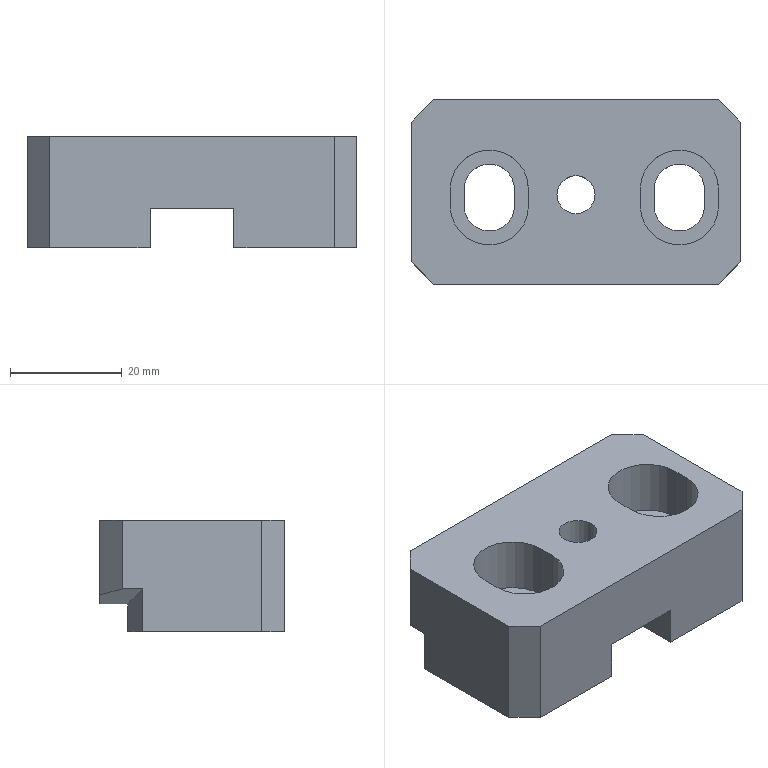Part | NX | features 20 2 | 1 solid | 41 faces | box 59 x 33 x 20 mm | volume 27333 mm3 | plane 32 | cylinder 9 | commonest cylinder face diameters 9 x4 14 x4 6.8 x1
STEP:
#1=CARTESIAN_POINT('',(2805.502,-433.5,16.5));
#2=VERTEX_POINT('',#1);
#3=CARTESIAN_POINT('',(2791.502,-433.5,16.5));
#4=VERTEX_POINT('',#3);
#5=CARTESIAN_POINT('',(2798.502,-433.5,16.5));
#6=DIRECTION('',(0.,0.,1.));
#7=DIRECTION('',(1.,0.,0.));
#8=AXIS2_PLACEMENT_3D('',#5,#6,#7);
#9=CIRCLE('',#8,7.);
#10=EDGE_CURVE('',#2,#4,#9,.T.);
#11=ORIENTED_EDGE('',*,*,#10,.F.);
#12=CARTESIAN_POINT('',(2805.502,-436.5,16.5));
#13=VERTEX_POINT('',#12);
#14=CARTESIAN_POINT('',(2805.502,-450.5,16.5));
#15=DIRECTION('',(0.,1.,0.));
#16=VECTOR('',#15,1000.);
#17=LINE('',#14,#16);
#18=EDGE_CURVE('',#13,#2,#17,.T.);
#19=ORIENTED_EDGE('',*,*,#18,.F.);
#20=CARTESIAN_POINT('',(2791.502,-436.5,16.5));
#21=VERTEX_POINT('',#20);
#22=CARTESIAN_POINT('',(2798.502,-436.5,16.5));
#23=DIRECTION('',(0.,0.,1.));
#24=DIRECTION('',(1.,0.,0.));
#25=AXIS2_PLACEMENT_3D('',#22,#23,#24);
#26=CIRCLE('',#25,7.);
#27=EDGE_CURVE('',#21,#13,#26,.T.);
#28=ORIENTED_EDGE('',*,*,#27,.F.);
#29=CARTESIAN_POINT('',(2791.502,-450.5,16.5));
#30=DIRECTION('',(0.,-1.,0.));
#31=VECTOR('',#30,1000.);
#32=LINE('',#29,#31);
#33=EDGE_CURVE('',#4,#21,#32,.T.);
#34=ORIENTED_EDGE('',*,*,#33,.F.);
#35=EDGE_LOOP('',(#11,#19,#28,#34));
#36=FACE_BOUND('',#35,.T.);
#37=CARTESIAN_POINT('',(2771.502,-436.5,16.5));
#38=VERTEX_POINT('',#37);
#39=CARTESIAN_POINT('',(2771.502,-433.5,16.5));
#40=VERTEX_POINT('',#39);
#41=CARTESIAN_POINT('',(2771.502,-450.5,16.5));
#42=DIRECTION('',(0.,1.,0.));
#43=VECTOR('',#42,1000.);
#44=LINE('',#41,#43);
#45=EDGE_CURVE('',#38,#40,#44,.T.);
#46=ORIENTED_EDGE('',*,*,#45,.F.);
#47=CARTESIAN_POINT('',(2757.502,-436.5,16.5));
#48=VERTEX_POINT('',#47);
#49=CARTESIAN_POINT('',(2764.502,-436.5,16.5));
#50=DIRECTION('',(0.,0.,1.));
#51=DIRECTION('',(1.,0.,0.));
#52=AXIS2_PLACEMENT_3D('',#49,#50,#51);
#53=CIRCLE('',#52,7.);
#54=EDGE_CURVE('',#48,#38,#53,.T.);
#55=ORIENTED_EDGE('',*,*,#54,.F.);
#56=CARTESIAN_POINT('',(2757.502,-433.5,16.5));
#57=VERTEX_POINT('',#56);
#58=CARTESIAN_POINT('',(2757.502,-450.5,16.5));
#59=DIRECTION('',(0.,-1.,0.));
#60=VECTOR('',#59,1000.);
#61=LINE('',#58,#60);
#62=EDGE_CURVE('',#57,#48,#61,.T.);
#63=ORIENTED_EDGE('',*,*,#62,.F.);
#64=CARTESIAN_POINT('',(2764.502,-433.5,16.5));
#65=DIRECTION('',(0.,0.,1.));
#66=DIRECTION('',(1.,0.,0.));
#67=AXIS2_PLACEMENT_3D('',#64,#65,#66);
#68=CIRCLE('',#67,7.);
#69=EDGE_CURVE('',#40,#57,#68,.T.);
#70=ORIENTED_EDGE('',*,*,#69,.F.);
#71=EDGE_LOOP('',(#46,#55,#63,#70));
#72=FACE_BOUND('',#71,.T.);
#73=CARTESIAN_POINT('',(2805.502,-417.5,16.5));
#74=VERTEX_POINT('',#73);
#75=CARTESIAN_POINT('',(2754.502,-417.5,16.5));
#76=VERTEX_POINT('',#75);
#77=CARTESIAN_POINT('',(2908.502,-417.5,16.5));
#78=DIRECTION('',(-1.,0.,0.));
#79=VECTOR('',#78,1000.);
#80=LINE('',#77,#79);
#81=EDGE_CURVE('',#74,#76,#80,.T.);
#82=ORIENTED_EDGE('',*,*,#81,.T.);
#83=CARTESIAN_POINT('',(2750.502,-421.5,16.5));
#84=VERTEX_POINT('',#83);
#85=CARTESIAN_POINT('',(2750.502,-421.5,16.5));
#86=DIRECTION('',(-0.7071,-0.7071,0.));
#87=VECTOR('',#86,1000.);
#88=LINE('',#85,#87);
#89=EDGE_CURVE('',#76,#84,#88,.T.);
#90=ORIENTED_EDGE('',*,*,#89,.T.);
#91=CARTESIAN_POINT('',(2750.502,-446.5,16.5));
#92=VERTEX_POINT('',#91);
#93=CARTESIAN_POINT('',(2750.502,-417.5,16.5));
#94=DIRECTION('',(0.,-1.,0.));
#95=VECTOR('',#94,1000.);
#96=LINE('',#93,#95);
#97=EDGE_CURVE('',#84,#92,#96,.T.);
#98=ORIENTED_EDGE('',*,*,#97,.T.);
#99=CARTESIAN_POINT('',(2754.502,-450.5,16.5));
#100=VERTEX_POINT('',#99);
#101=CARTESIAN_POINT('',(2754.502,-450.5,16.5));
#102=DIRECTION('',(0.7071,-0.7071,0.));
#103=VECTOR('',#102,1000.);
#104=LINE('',#101,#103);
#105=EDGE_CURVE('',#92,#100,#104,.T.);
#106=ORIENTED_EDGE('',*,*,#105,.T.);
#107=CARTESIAN_POINT('',(2805.502,-450.5,16.5));
#108=VERTEX_POINT('',#107);
#109=CARTESIAN_POINT('',(2828.502,-450.5,16.5));
#110=DIRECTION('',(1.,0.,0.));
#111=VECTOR('',#110,1000.);
#112=LINE('',#109,#111);
#113=EDGE_CURVE('',#100,#108,#112,.T.);
#114=ORIENTED_EDGE('',*,*,#113,.T.);
#115=CARTESIAN_POINT('',(2809.502,-446.5,16.5));
#116=VERTEX_POINT('',#115);
#117=CARTESIAN_POINT('',(2809.502,-446.5,16.5));
#118=DIRECTION('',(0.7071,0.7071,0.));
#119=VECTOR('',#118,1000.);
#120=LINE('',#117,#119);
#121=EDGE_CURVE('',#108,#116,#120,.T.);
#122=ORIENTED_EDGE('',*,*,#121,.T.);
#123=CARTESIAN_POINT('',(2809.502,-421.5,16.5));
#124=VERTEX_POINT('',#123);
#125=CARTESIAN_POINT('',(2809.502,-450.5,16.5));
#126=DIRECTION('',(0.,1.,0.));
#127=VECTOR('',#126,1000.);
#128=LINE('',#125,#127);
#129=EDGE_CURVE('',#116,#124,#128,.T.);
#130=ORIENTED_EDGE('',*,*,#129,.T.);
#131=CARTESIAN_POINT('',(2805.502,-417.5,16.5));
#132=DIRECTION('',(-0.7071,0.7071,0.));
#133=VECTOR('',#132,1000.);
#134=LINE('',#131,#133);
#135=EDGE_CURVE('',#124,#74,#134,.T.);
#136=ORIENTED_EDGE('',*,*,#135,.T.);
#137=EDGE_LOOP('',(#82,#90,#98,#106,#114,#122,#130,#136));
#138=FACE_BOUND('',#137,.T.);
#139=CARTESIAN_POINT('',(2783.402,-434.5,16.5));
#140=VERTEX_POINT('',#139);
#141=CARTESIAN_POINT('',(2780.002,-434.5,16.5));
#142=DIRECTION('',(0.,0.,-1.));
#143=DIRECTION('',(1.,0.,0.));
#144=AXIS2_PLACEMENT_3D('',#141,#142,#143);
#145=CIRCLE('',#144,3.4);
#146=EDGE_CURVE('',#140,#140,#145,.T.);
#147=ORIENTED_EDGE('',*,*,#146,.T.);
#148=EDGE_LOOP('',(#147));
#149=FACE_BOUND('',#148,.T.);
#150=CARTESIAN_POINT('',(2908.502,-450.5,16.5));
#151=DIRECTION('',(0.,0.,1.));
#152=DIRECTION('',(-1.,0.,0.));
#153=AXIS2_PLACEMENT_3D('',#150,#151,#152);
#154=PLANE('',#153);
#155=ADVANCED_FACE('',(#36,#72,#138,#149),#154,.T.);
#156=CARTESIAN_POINT('',(2787.502,-417.5,3.5));
#157=VERTEX_POINT('',#156);
#158=CARTESIAN_POINT('',(2787.502,-450.5,3.5));
#159=VERTEX_POINT('',#158);
#160=CARTESIAN_POINT('',(2787.502,-436.5,3.5));
#161=DIRECTION('',(0.,-1.,0.));
#162=VECTOR('',#161,1000.);
#163=LINE('',#160,#162);
#164=EDGE_CURVE('',#157,#159,#163,.T.);
#165=ORIENTED_EDGE('',*,*,#164,.F.);
#166=CARTESIAN_POINT('',(2787.502,-417.5,1.5));
#167=VERTEX_POINT('',#166);
#168=CARTESIAN_POINT('',(2787.502,-417.5,11.5));
#169=DIRECTION('',(0.,0.,-1.));
#170=VECTOR('',#169,1000.);
#171=LINE('',#168,#170);
#172=EDGE_CURVE('',#157,#167,#171,.T.);
#173=ORIENTED_EDGE('',*,*,#172,.T.);
#174=CARTESIAN_POINT('',(2787.502,-422.5,1.5));
#175=VERTEX_POINT('',#174);
#176=CARTESIAN_POINT('',(2787.502,-396.891,1.5));
#177=DIRECTION('',(0.,1.,0.));
#178=VECTOR('',#177,1000.);
#179=LINE('',#176,#178);
#180=EDGE_CURVE('',#175,#167,#179,.T.);
#181=ORIENTED_EDGE('',*,*,#180,.F.);
#182=CARTESIAN_POINT('',(2787.502,-422.5,-3.5));
#183=VERTEX_POINT('',#182);
#184=CARTESIAN_POINT('',(2787.502,-422.5,3.5));
#185=DIRECTION('',(0.,0.,-1.));
#186=VECTOR('',#185,1000.);
#187=LINE('',#184,#186);
#188=EDGE_CURVE('',#175,#183,#187,.T.);
#189=ORIENTED_EDGE('',*,*,#188,.T.);
#190=CARTESIAN_POINT('',(2787.502,-450.5,-3.5));
#191=VERTEX_POINT('',#190);
#192=CARTESIAN_POINT('',(2787.502,-450.5,-3.5));
#193=DIRECTION('',(0.,-1.,0.));
#194=VECTOR('',#193,1000.);
#195=LINE('',#192,#194);
#196=EDGE_CURVE('',#183,#191,#195,.T.);
#197=ORIENTED_EDGE('',*,*,#196,.T.);
#198=CARTESIAN_POINT('',(2787.502,-450.5,11.5));
#199=DIRECTION('',(0.,0.,1.));
#200=VECTOR('',#199,1000.);
#201=LINE('',#198,#200);
#202=EDGE_CURVE('',#191,#159,#201,.T.);
#203=ORIENTED_EDGE('',*,*,#202,.T.);
#204=EDGE_LOOP('',(#165,#173,#181,#189,#197,#203));
#205=FACE_BOUND('',#204,.T.);
#206=CARTESIAN_POINT('',(2787.502,-436.5,0.));
#207=DIRECTION('',(-1.,0.,0.));
#208=DIRECTION('',(0.,0.,1.));
#209=AXIS2_PLACEMENT_3D('',#206,#207,#208);
#210=PLANE('',#209);
#211=ADVANCED_FACE('',(#205),#210,.T.);
#212=CARTESIAN_POINT('',(2772.502,-422.5,-3.5));
#213=VERTEX_POINT('',#212);
#214=CARTESIAN_POINT('',(2772.502,-450.5,-3.5));
#215=VERTEX_POINT('',#214);
#216=CARTESIAN_POINT('',(2772.502,-450.5,-3.5));
#217=DIRECTION('',(0.,-1.,0.));
#218=VECTOR('',#217,1000.);
#219=LINE('',#216,#218);
#220=EDGE_CURVE('',#213,#215,#219,.T.);
#221=ORIENTED_EDGE('',*,*,#220,.F.);
#222=CARTESIAN_POINT('',(2772.502,-422.5,1.5));
#223=VERTEX_POINT('',#222);
#224=CARTESIAN_POINT('',(2772.502,-422.5,3.5));
#225=DIRECTION('',(0.,0.,-1.));
#226=VECTOR('',#225,1000.);
#227=LINE('',#224,#226);
#228=EDGE_CURVE('',#223,#213,#227,.T.);
#229=ORIENTED_EDGE('',*,*,#228,.F.);
#230=CARTESIAN_POINT('',(2772.502,-417.5,1.5));
#231=VERTEX_POINT('',#230);
#232=CARTESIAN_POINT('',(2772.502,-396.891,1.5));
#233=DIRECTION('',(0.,1.,0.));
#234=VECTOR('',#233,1000.);
#235=LINE('',#232,#234);
#236=EDGE_CURVE('',#223,#231,#235,.T.);
#237=ORIENTED_EDGE('',*,*,#236,.T.);
#238=CARTESIAN_POINT('',(2772.502,-417.5,3.5));
#239=VERTEX_POINT('',#238);
#240=CARTESIAN_POINT('',(2772.502,-417.5,11.5));
#241=DIRECTION('',(0.,0.,-1.));
#242=VECTOR('',#241,1000.);
#243=LINE('',#240,#242);
#244=EDGE_CURVE('',#239,#231,#243,.T.);
#245=ORIENTED_EDGE('',*,*,#244,.F.);
#246=CARTESIAN_POINT('',(2772.502,-450.5,3.5));
#247=VERTEX_POINT('',#246);
#248=CARTESIAN_POINT('',(2772.502,-436.5,3.5));
#249=DIRECTION('',(0.,1.,0.));
#250=VECTOR('',#249,1000.);
#251=LINE('',#248,#250);
#252=EDGE_CURVE('',#247,#239,#251,.T.);
#253=ORIENTED_EDGE('',*,*,#252,.F.);
#254=CARTESIAN_POINT('',(2772.502,-450.5,11.5));
#255=DIRECTION('',(0.,0.,1.));
#256=VECTOR('',#255,1000.);
#257=LINE('',#254,#256);
#258=EDGE_CURVE('',#215,#247,#257,.T.);
#259=ORIENTED_EDGE('',*,*,#258,.F.);
#260=EDGE_LOOP('',(#221,#229,#237,#245,#253,#259));
#261=FACE_BOUND('',#260,.T.);
#262=CARTESIAN_POINT('',(2772.502,-436.5,-9.5));
#263=DIRECTION('',(-1.,0.,0.));
#264=DIRECTION('',(0.,0.,-1.));
#265=AXIS2_PLACEMENT_3D('',#262,#263,#264);
#266=PLANE('',#265);
#267=ADVANCED_FACE('',(#261),#266,.F.);
#268=CARTESIAN_POINT('',(2783.402,-434.5,3.5));
#269=VERTEX_POINT('',#268);
#270=CARTESIAN_POINT('',(2780.002,-434.5,3.5));
#271=DIRECTION('',(0.,0.,1.));
#272=DIRECTION('',(1.,0.,0.));
#273=AXIS2_PLACEMENT_3D('',#270,#271,#272);
#274=CIRCLE('',#273,3.4);
#275=EDGE_CURVE('',#269,#269,#274,.T.);
#276=ORIENTED_EDGE('',*,*,#275,.T.);
#277=EDGE_LOOP('',(#276));
#278=FACE_BOUND('',#277,.T.);
#279=CARTESIAN_POINT('',(2850.502,-450.5,3.5));
#280=DIRECTION('',(1.,0.,0.));
#281=VECTOR('',#280,1000.);
#282=LINE('',#279,#281);
#283=EDGE_CURVE('',#247,#159,#282,.T.);
#284=ORIENTED_EDGE('',*,*,#283,.F.);
#285=ORIENTED_EDGE('',*,*,#252,.T.);
#286=CARTESIAN_POINT('',(2930.502,-417.5,3.5));
#287=DIRECTION('',(-1.,0.,0.));
#288=VECTOR('',#287,1000.);
#289=LINE('',#286,#288);
#290=EDGE_CURVE('',#157,#239,#289,.T.);
#291=ORIENTED_EDGE('',*,*,#290,.F.);
#292=ORIENTED_EDGE('',*,*,#164,.T.);
#293=EDGE_LOOP('',(#284,#285,#291,#292));
#294=FACE_BOUND('',#293,.T.);
#295=CARTESIAN_POINT('',(2780.002,-436.5,3.5));
#296=DIRECTION('',(0.,0.,1.));
#297=DIRECTION('',(0.,-1.,0.));
#298=AXIS2_PLACEMENT_3D('',#295,#296,#297);
#299=PLANE('',#298);
#300=ADVANCED_FACE('',(#278,#294),#299,.F.);
#301=CARTESIAN_POINT('',(2794.002,-436.5,6.5));
#302=VERTEX_POINT('',#301);
#303=CARTESIAN_POINT('',(2794.002,-433.5,6.5));
#304=VERTEX_POINT('',#303);
#305=CARTESIAN_POINT('',(2794.002,-432.5,6.5));
#306=DIRECTION('',(0.,1.,0.));
#307=VECTOR('',#306,1000.);
#308=LINE('',#305,#307);
#309=EDGE_CURVE('',#302,#304,#308,.T.);
#310=ORIENTED_EDGE('',*,*,#309,.T.);
#311=CARTESIAN_POINT('',(2803.002,-433.5,6.5));
#312=VERTEX_POINT('',#311);
#313=CARTESIAN_POINT('',(2798.502,-433.5,6.5));
#314=DIRECTION('',(0.,0.,-1.));
#315=DIRECTION('',(-1.,0.,0.));
#316=AXIS2_PLACEMENT_3D('',#313,#314,#315);
#317=CIRCLE('',#316,4.5);
#318=EDGE_CURVE('',#304,#312,#317,.T.);
#319=ORIENTED_EDGE('',*,*,#318,.T.);
#320=CARTESIAN_POINT('',(2803.002,-436.5,6.5));
#321=VERTEX_POINT('',#320);
#322=CARTESIAN_POINT('',(2803.002,-439.5,6.5));
#323=DIRECTION('',(0.,-1.,0.));
#324=VECTOR('',#323,1000.);
#325=LINE('',#322,#324);
#326=EDGE_CURVE('',#312,#321,#325,.T.);
#327=ORIENTED_EDGE('',*,*,#326,.T.);
#328=CARTESIAN_POINT('',(2798.502,-436.5,6.5));
#329=DIRECTION('',(0.,0.,-1.));
#330=DIRECTION('',(-1.,0.,0.));
#331=AXIS2_PLACEMENT_3D('',#328,#329,#330);
#332=CIRCLE('',#331,4.5);
#333=EDGE_CURVE('',#321,#302,#332,.T.);
#334=ORIENTED_EDGE('',*,*,#333,.T.);
#335=EDGE_LOOP('',(#310,#319,#327,#334));
#336=FACE_BOUND('',#335,.T.);
#337=CARTESIAN_POINT('',(2805.502,-433.5,6.5));
#338=VERTEX_POINT('',#337);
#339=CARTESIAN_POINT('',(2791.502,-433.5,6.5));
#340=VERTEX_POINT('',#339);
#341=CARTESIAN_POINT('',(2798.502,-433.5,6.5));
#342=DIRECTION('',(0.,0.,1.));
#343=DIRECTION('',(-1.,0.,0.));
#344=AXIS2_PLACEMENT_3D('',#341,#342,#343);
#345=CIRCLE('',#344,7.);
#346=EDGE_CURVE('',#338,#340,#345,.T.);
#347=ORIENTED_EDGE('',*,*,#346,.T.);
#348=CARTESIAN_POINT('',(2791.502,-436.5,6.5));
#349=VERTEX_POINT('',#348);
#350=CARTESIAN_POINT('',(2791.502,-439.5,6.5));
#351=DIRECTION('',(0.,-1.,0.));
#352=VECTOR('',#351,1000.);
#353=LINE('',#350,#352);
#354=EDGE_CURVE('',#340,#349,#353,.T.);
#355=ORIENTED_EDGE('',*,*,#354,.T.);
#356=CARTESIAN_POINT('',(2805.502,-436.5,6.5));
#357=VERTEX_POINT('',#356);
#358=CARTESIAN_POINT('',(2798.502,-436.5,6.5));
#359=DIRECTION('',(0.,0.,1.));
#360=DIRECTION('',(-1.,0.,0.));
#361=AXIS2_PLACEMENT_3D('',#358,#359,#360);
#362=CIRCLE('',#361,7.);
#363=EDGE_CURVE('',#349,#357,#362,.T.);
#364=ORIENTED_EDGE('',*,*,#363,.T.);
#365=CARTESIAN_POINT('',(2805.502,-432.5,6.5));
#366=DIRECTION('',(0.,1.,0.));
#367=VECTOR('',#366,1000.);
#368=LINE('',#365,#367);
#369=EDGE_CURVE('',#357,#338,#368,.T.);
#370=ORIENTED_EDGE('',*,*,#369,.T.);
#371=EDGE_LOOP('',(#347,#355,#364,#370));
#372=FACE_BOUND('',#371,.T.);
#373=CARTESIAN_POINT('',(2798.502,-432.5,6.5));
#374=DIRECTION('',(0.,0.,-1.));
#375=DIRECTION('',(1.,0.,0.));
#376=AXIS2_PLACEMENT_3D('',#373,#374,#375);
#377=PLANE('',#376);
#378=ADVANCED_FACE('',(#336,#372),#377,.F.);
#379=CARTESIAN_POINT('',(2799.502,-417.5,1.5));
#380=VERTEX_POINT('',#379);
#381=CARTESIAN_POINT('',(2799.502,-422.5,1.5));
#382=VERTEX_POINT('',#381);
#383=CARTESIAN_POINT('',(2799.502,-425.18,1.5));
#384=DIRECTION('',(0.,-1.,0.));
#385=VECTOR('',#384,1000.);
#386=LINE('',#383,#385);
#387=EDGE_CURVE('',#380,#382,#386,.T.);
#388=ORIENTED_EDGE('',*,*,#387,.F.);
#389=CARTESIAN_POINT('',(2805.502,-417.5,3.108));
#390=VERTEX_POINT('',#389);
#391=CARTESIAN_POINT('',(2799.502,-417.5,1.5));
#392=DIRECTION('',(-0.9659,0.,-0.2588));
#393=VECTOR('',#392,1000.);
#394=LINE('',#391,#393);
#395=EDGE_CURVE('',#390,#380,#394,.T.);
#396=ORIENTED_EDGE('',*,*,#395,.F.);
#397=CARTESIAN_POINT('',(2809.502,-421.5,4.179));
#398=VERTEX_POINT('',#397);
#399=CARTESIAN_POINT('',(2792.451,-404.449,-0.3894));
#400=DIRECTION('',(0.6947,-0.6947,0.1862));
#401=VECTOR('',#400,1000.);
#402=LINE('',#399,#401);
#403=EDGE_CURVE('',#390,#398,#402,.T.);
#404=ORIENTED_EDGE('',*,*,#403,.T.);
#405=CARTESIAN_POINT('',(2809.502,-425.18,4.179));
#406=VERTEX_POINT('',#405);
#407=CARTESIAN_POINT('',(2809.502,-417.5,4.179));
#408=DIRECTION('',(0.,1.,0.));
#409=VECTOR('',#408,1000.);
#410=LINE('',#407,#409);
#411=EDGE_CURVE('',#406,#398,#410,.T.);
#412=ORIENTED_EDGE('',*,*,#411,.F.);
#413=CARTESIAN_POINT('',(2808.875,-425.012,4.011));
#414=DIRECTION('',(0.9351,-0.2506,0.2506));
#415=VECTOR('',#414,1000.);
#416=LINE('',#413,#415);
#417=EDGE_CURVE('',#382,#406,#416,.T.);
#418=ORIENTED_EDGE('',*,*,#417,.F.);
#419=EDGE_LOOP('',(#388,#396,#404,#412,#418));
#420=FACE_BOUND('',#419,.T.);
#421=CARTESIAN_POINT('',(2799.502,-396.891,1.5));
#422=DIRECTION('',(0.2588,0.,-0.9659));
#423=DIRECTION('',(0.9659,0.,0.2588));
#424=AXIS2_PLACEMENT_3D('',#421,#422,#423);
#425=PLANE('',#424);
#426=ADVANCED_FACE('',(#420),#425,.T.);
#427=CARTESIAN_POINT('',(2769.002,-433.5,6.5));
#428=VERTEX_POINT('',#427);
#429=CARTESIAN_POINT('',(2769.002,-436.5,6.5));
#430=VERTEX_POINT('',#429);
#431=CARTESIAN_POINT('',(2769.002,-432.5,6.5));
#432=DIRECTION('',(0.,-1.,0.));
#433=VECTOR('',#432,1000.);
#434=LINE('',#431,#433);
#435=EDGE_CURVE('',#428,#430,#434,.T.);
#436=ORIENTED_EDGE('',*,*,#435,.T.);
#437=CARTESIAN_POINT('',(2760.002,-436.5,6.5));
#438=VERTEX_POINT('',#437);
#439=CARTESIAN_POINT('',(2764.502,-436.5,6.5));
#440=DIRECTION('',(0.,0.,-1.));
#441=DIRECTION('',(-1.,0.,0.));
#442=AXIS2_PLACEMENT_3D('',#439,#440,#441);
#443=CIRCLE('',#442,4.5);
#444=EDGE_CURVE('',#430,#438,#443,.T.);
#445=ORIENTED_EDGE('',*,*,#444,.T.);
#446=CARTESIAN_POINT('',(2760.002,-433.5,6.5));
#447=VERTEX_POINT('',#446);
#448=CARTESIAN_POINT('',(2760.002,-439.5,6.5));
#449=DIRECTION('',(0.,1.,0.));
#450=VECTOR('',#449,1000.);
#451=LINE('',#448,#450);
#452=EDGE_CURVE('',#438,#447,#451,.T.);
#453=ORIENTED_EDGE('',*,*,#452,.T.);
#454=CARTESIAN_POINT('',(2764.502,-433.5,6.5));
#455=DIRECTION('',(0.,0.,-1.));
#456=DIRECTION('',(-1.,0.,0.));
#457=AXIS2_PLACEMENT_3D('',#454,#455,#456);
#458=CIRCLE('',#457,4.5);
#459=EDGE_CURVE('',#447,#428,#458,.T.);
#460=ORIENTED_EDGE('',*,*,#459,.T.);
#461=EDGE_LOOP('',(#436,#445,#453,#460));
#462=FACE_BOUND('',#461,.T.);
#463=CARTESIAN_POINT('',(2771.502,-433.5,6.5));
#464=VERTEX_POINT('',#463);
#465=CARTESIAN_POINT('',(2757.502,-433.5,6.5));
#466=VERTEX_POINT('',#465);
#467=CARTESIAN_POINT('',(2764.502,-433.5,6.5));
#468=DIRECTION('',(0.,0.,1.));
#469=DIRECTION('',(-1.,0.,0.));
#470=AXIS2_PLACEMENT_3D('',#467,#468,#469);
#471=CIRCLE('',#470,7.);
#472=EDGE_CURVE('',#464,#466,#471,.T.);
#473=ORIENTED_EDGE('',*,*,#472,.T.);
#474=CARTESIAN_POINT('',(2757.502,-436.5,6.5));
#475=VERTEX_POINT('',#474);
#476=CARTESIAN_POINT('',(2757.502,-432.5,6.5));
#477=DIRECTION('',(0.,-1.,0.));
#478=VECTOR('',#477,1000.);
#479=LINE('',#476,#478);
#480=EDGE_CURVE('',#466,#475,#479,.T.);
#481=ORIENTED_EDGE('',*,*,#480,.T.);
#482=CARTESIAN_POINT('',(2771.502,-436.5,6.5));
#483=VERTEX_POINT('',#482);
#484=CARTESIAN_POINT('',(2764.502,-436.5,6.5));
#485=DIRECTION('',(0.,0.,1.));
#486=DIRECTION('',(-1.,0.,0.));
#487=AXIS2_PLACEMENT_3D('',#484,#485,#486);
#488=CIRCLE('',#487,7.);
#489=EDGE_CURVE('',#475,#483,#488,.T.);
#490=ORIENTED_EDGE('',*,*,#489,.T.);
#491=CARTESIAN_POINT('',(2771.502,-439.5,6.5));
#492=DIRECTION('',(0.,1.,0.));
#493=VECTOR('',#492,1000.);
#494=LINE('',#491,#493);
#495=EDGE_CURVE('',#483,#464,#494,.T.);
#496=ORIENTED_EDGE('',*,*,#495,.T.);
#497=EDGE_LOOP('',(#473,#481,#490,#496));
#498=FACE_BOUND('',#497,.T.);
#499=CARTESIAN_POINT('',(2764.502,-432.5,6.5));
#500=DIRECTION('',(0.,0.,-1.));
#501=DIRECTION('',(-1.,0.,0.));
#502=AXIS2_PLACEMENT_3D('',#499,#500,#501);
#503=PLANE('',#502);
#504=ADVANCED_FACE('',(#462,#498),#503,.F.);
#505=ORIENTED_EDGE('',*,*,#33,.T.);
#506=CARTESIAN_POINT('',(2791.502,-436.5,42.5));
#507=DIRECTION('',(0.,0.,1.));
#508=VECTOR('',#507,1000.);
#509=LINE('',#506,#508);
#510=EDGE_CURVE('',#349,#21,#509,.T.);
#511=ORIENTED_EDGE('',*,*,#510,.F.);
#512=ORIENTED_EDGE('',*,*,#354,.F.);
#513=CARTESIAN_POINT('',(2791.502,-433.5,42.5));
#514=DIRECTION('',(0.,0.,1.));
#515=VECTOR('',#514,1000.);
#516=LINE('',#513,#515);
#517=EDGE_CURVE('',#340,#4,#516,.T.);
#518=ORIENTED_EDGE('',*,*,#517,.T.);
#519=EDGE_LOOP('',(#505,#511,#512,#518));
#520=FACE_BOUND('',#519,.T.);
#521=CARTESIAN_POINT('',(2791.502,-439.5,42.5));
#522=DIRECTION('',(-1.,0.,0.));
#523=DIRECTION('',(0.,0.,-1.));
#524=AXIS2_PLACEMENT_3D('',#521,#522,#523);
#525=PLANE('',#524);
#526=ADVANCED_FACE('',(#520),#525,.F.);
#527=ORIENTED_EDGE('',*,*,#27,.T.);
#528=CARTESIAN_POINT('',(2805.502,-436.5,42.5));
#529=DIRECTION('',(0.,0.,1.));
#530=VECTOR('',#529,1000.);
#531=LINE('',#528,#530);
#532=EDGE_CURVE('',#357,#13,#531,.T.);
#533=ORIENTED_EDGE('',*,*,#532,.F.);
#534=ORIENTED_EDGE('',*,*,#363,.F.);
#535=ORIENTED_EDGE('',*,*,#510,.T.);
#536=EDGE_LOOP('',(#527,#533,#534,#535));
#537=FACE_BOUND('',#536,.T.);
#538=CARTESIAN_POINT('',(2798.502,-436.5,42.5));
#539=DIRECTION('',(0.,0.,-1.));
#540=DIRECTION('',(1.,0.,0.));
#541=AXIS2_PLACEMENT_3D('',#538,#539,#540);
#542=CYLINDRICAL_SURFACE('',#541,7.);
#543=ADVANCED_FACE('',(#537),#542,.F.);
#544=ORIENTED_EDGE('',*,*,#18,.T.);
#545=CARTESIAN_POINT('',(2805.502,-433.5,42.5));
#546=DIRECTION('',(0.,0.,1.));
#547=VECTOR('',#546,1000.);
#548=LINE('',#545,#547);
#549=EDGE_CURVE('',#338,#2,#548,.T.);
#550=ORIENTED_EDGE('',*,*,#549,.F.);
#551=ORIENTED_EDGE('',*,*,#369,.F.);
#552=ORIENTED_EDGE('',*,*,#532,.T.);
#553=EDGE_LOOP('',(#544,#550,#551,#552));
#554=FACE_BOUND('',#553,.T.);
#555=CARTESIAN_POINT('',(2805.502,-432.5,42.5));
#556=DIRECTION('',(1.,0.,0.));
#557=DIRECTION('',(0.,0.,1.));
#558=AXIS2_PLACEMENT_3D('',#555,#556,#557);
#559=PLANE('',#558);
#560=ADVANCED_FACE('',(#554),#559,.F.);
#561=ORIENTED_EDGE('',*,*,#10,.T.);
#562=ORIENTED_EDGE('',*,*,#517,.F.);
#563=ORIENTED_EDGE('',*,*,#346,.F.);
#564=ORIENTED_EDGE('',*,*,#549,.T.);
#565=EDGE_LOOP('',(#561,#562,#563,#564));
#566=FACE_BOUND('',#565,.T.);
#567=CARTESIAN_POINT('',(2798.502,-433.5,42.5));
#568=DIRECTION('',(0.,0.,-1.));
#569=DIRECTION('',(1.,0.,0.));
#570=AXIS2_PLACEMENT_3D('',#567,#568,#569);
#571=CYLINDRICAL_SURFACE('',#570,7.);
#572=ADVANCED_FACE('',(#566),#571,.F.);
#573=ORIENTED_EDGE('',*,*,#135,.F.);
#574=CARTESIAN_POINT('',(2809.502,-421.5,11.5));
#575=DIRECTION('',(0.,0.,1.));
#576=VECTOR('',#575,1000.);
#577=LINE('',#574,#576);
#578=EDGE_CURVE('',#398,#124,#577,.T.);
#579=ORIENTED_EDGE('',*,*,#578,.F.);
#580=ORIENTED_EDGE('',*,*,#403,.F.);
#581=CARTESIAN_POINT('',(2805.502,-417.5,11.5));
#582=DIRECTION('',(0.,0.,-1.));
#583=VECTOR('',#582,1000.);
#584=LINE('',#581,#583);
#585=EDGE_CURVE('',#74,#390,#584,.T.);
#586=ORIENTED_EDGE('',*,*,#585,.F.);
#587=EDGE_LOOP('',(#573,#579,#580,#586));
#588=FACE_BOUND('',#587,.T.);
#589=CARTESIAN_POINT('',(2805.502,-417.5,11.5));
#590=DIRECTION('',(-0.7071,-0.7071,0.));
#591=DIRECTION('',(0.,0.,-1.));
#592=AXIS2_PLACEMENT_3D('',#589,#590,#591);
#593=PLANE('',#592);
#594=ADVANCED_FACE('',(#588),#593,.F.);
#595=ORIENTED_EDGE('',*,*,#69,.T.);
#596=CARTESIAN_POINT('',(2757.502,-433.5,42.5));
#597=DIRECTION('',(0.,0.,-1.));
#598=VECTOR('',#597,1000.);
#599=LINE('',#596,#598);
#600=EDGE_CURVE('',#57,#466,#599,.T.);
#601=ORIENTED_EDGE('',*,*,#600,.T.);
#602=ORIENTED_EDGE('',*,*,#472,.F.);
#603=CARTESIAN_POINT('',(2771.502,-433.5,42.5));
#604=DIRECTION('',(0.,0.,-1.));
#605=VECTOR('',#604,1000.);
#606=LINE('',#603,#605);
#607=EDGE_CURVE('',#40,#464,#606,.T.);
#608=ORIENTED_EDGE('',*,*,#607,.F.);
#609=EDGE_LOOP('',(#595,#601,#602,#608));
#610=FACE_BOUND('',#609,.T.);
#611=CARTESIAN_POINT('',(2764.502,-433.5,42.5));
#612=DIRECTION('',(0.,0.,-1.));
#613=DIRECTION('',(-1.,0.,0.));
#614=AXIS2_PLACEMENT_3D('',#611,#612,#613);
#615=CYLINDRICAL_SURFACE('',#614,7.);
#616=ADVANCED_FACE('',(#610),#615,.F.);
#617=ORIENTED_EDGE('',*,*,#62,.T.);
#618=CARTESIAN_POINT('',(2757.502,-436.5,42.5));
#619=DIRECTION('',(0.,0.,-1.));
#620=VECTOR('',#619,1000.);
#621=LINE('',#618,#620);
#622=EDGE_CURVE('',#48,#475,#621,.T.);
#623=ORIENTED_EDGE('',*,*,#622,.T.);
#624=ORIENTED_EDGE('',*,*,#480,.F.);
#625=ORIENTED_EDGE('',*,*,#600,.F.);
#626=EDGE_LOOP('',(#617,#623,#624,#625));
#627=FACE_BOUND('',#626,.T.);
#628=CARTESIAN_POINT('',(2757.502,-432.5,42.5));
#629=DIRECTION('',(-1.,0.,0.));
#630=DIRECTION('',(0.,0.,1.));
#631=AXIS2_PLACEMENT_3D('',#628,#629,#630);
#632=PLANE('',#631);
#633=ADVANCED_FACE('',(#627),#632,.F.);
#634=ORIENTED_EDGE('',*,*,#54,.T.);
#635=CARTESIAN_POINT('',(2771.502,-436.5,42.5));
#636=DIRECTION('',(0.,0.,-1.));
#637=VECTOR('',#636,1000.);
#638=LINE('',#635,#637);
#639=EDGE_CURVE('',#38,#483,#638,.T.);
#640=ORIENTED_EDGE('',*,*,#639,.T.);
#641=ORIENTED_EDGE('',*,*,#489,.F.);
#642=ORIENTED_EDGE('',*,*,#622,.F.);
#643=EDGE_LOOP('',(#634,#640,#641,#642));
#644=FACE_BOUND('',#643,.T.);
#645=CARTESIAN_POINT('',(2764.502,-436.5,42.5));
#646=DIRECTION('',(0.,0.,-1.));
#647=DIRECTION('',(-1.,0.,0.));
#648=AXIS2_PLACEMENT_3D('',#645,#646,#647);
#649=CYLINDRICAL_SURFACE('',#648,7.);
#650=ADVANCED_FACE('',(#644),#649,.F.);
#651=ORIENTED_EDGE('',*,*,#45,.T.);
#652=ORIENTED_EDGE('',*,*,#607,.T.);
#653=ORIENTED_EDGE('',*,*,#495,.F.);
#654=ORIENTED_EDGE('',*,*,#639,.F.);
#655=EDGE_LOOP('',(#651,#652,#653,#654));
#656=FACE_BOUND('',#655,.T.);
#657=CARTESIAN_POINT('',(2771.502,-439.5,42.5));
#658=DIRECTION('',(1.,0.,0.));
#659=DIRECTION('',(0.,0.,-1.));
#660=AXIS2_PLACEMENT_3D('',#657,#658,#659);
#661=PLANE('',#660);
#662=ADVANCED_FACE('',(#656),#661,.F.);
#663=ORIENTED_EDGE('',*,*,#411,.T.);
#664=ORIENTED_EDGE('',*,*,#578,.T.);
#665=ORIENTED_EDGE('',*,*,#129,.F.);
#666=CARTESIAN_POINT('',(2809.502,-446.5,-3.5));
#667=VERTEX_POINT('',#666);
#668=CARTESIAN_POINT('',(2809.502,-446.5,11.5));
#669=DIRECTION('',(0.,0.,-1.));
#670=VECTOR('',#669,1000.);
#671=LINE('',#668,#670);
#672=EDGE_CURVE('',#116,#667,#671,.T.);
#673=ORIENTED_EDGE('',*,*,#672,.T.);
#674=CARTESIAN_POINT('',(2809.502,-425.18,-3.5));
#675=VERTEX_POINT('',#674);
#676=CARTESIAN_POINT('',(2809.502,-450.5,-3.5));
#677=DIRECTION('',(0.,1.,0.));
#678=VECTOR('',#677,1000.);
#679=LINE('',#676,#678);
#680=EDGE_CURVE('',#667,#675,#679,.T.);
#681=ORIENTED_EDGE('',*,*,#680,.T.);
#682=CARTESIAN_POINT('',(2809.502,-425.18,3.5));
#683=DIRECTION('',(0.,0.,-1.));
#684=VECTOR('',#683,1000.);
#685=LINE('',#682,#684);
#686=EDGE_CURVE('',#406,#675,#685,.T.);
#687=ORIENTED_EDGE('',*,*,#686,.F.);
#688=EDGE_LOOP('',(#663,#664,#665,#673,#681,#687));
#689=FACE_BOUND('',#688,.T.);
#690=CARTESIAN_POINT('',(2809.502,-450.5,11.5));
#691=DIRECTION('',(-1.,0.,0.));
#692=DIRECTION('',(0.,0.,-1.));
#693=AXIS2_PLACEMENT_3D('',#690,#691,#692);
#694=PLANE('',#693);
#695=ADVANCED_FACE('',(#689),#694,.F.);
#696=CARTESIAN_POINT('',(2799.501,-422.5,1.5));
#697=VERTEX_POINT('',#696);
#698=CARTESIAN_POINT('',(2809.502,-425.18,1.5));
#699=DIRECTION('',(0.9659,-0.2588,0.));
#700=VECTOR('',#699,1000.);
#701=LINE('',#698,#700);
#702=EDGE_CURVE('',#697,#382,#701,.T.);
#703=ORIENTED_EDGE('',*,*,#702,.T.);
#704=ORIENTED_EDGE('',*,*,#417,.T.);
#705=ORIENTED_EDGE('',*,*,#686,.T.);
#706=CARTESIAN_POINT('',(2799.501,-422.5,-3.5));
#707=VERTEX_POINT('',#706);
#708=CARTESIAN_POINT('',(2809.502,-425.18,-3.5));
#709=DIRECTION('',(-0.9659,0.2588,0.));
#710=VECTOR('',#709,1000.);
#711=LINE('',#708,#710);
#712=EDGE_CURVE('',#675,#707,#711,.T.);
#713=ORIENTED_EDGE('',*,*,#712,.T.);
#714=CARTESIAN_POINT('',(2799.501,-422.5,3.5));
#715=DIRECTION('',(0.,0.,1.));
#716=VECTOR('',#715,1000.);
#717=LINE('',#714,#716);
#718=EDGE_CURVE('',#707,#697,#717,.T.);
#719=ORIENTED_EDGE('',*,*,#718,.T.);
#720=EDGE_LOOP('',(#703,#704,#705,#713,#719));
#721=FACE_BOUND('',#720,.T.);
#722=CARTESIAN_POINT('',(2809.502,-425.18,3.5));
#723=DIRECTION('',(-0.2588,-0.9659,0.));
#724=DIRECTION('',(0.9659,-0.2588,0.));
#725=AXIS2_PLACEMENT_3D('',#722,#723,#724);
#726=PLANE('',#725);
#727=ADVANCED_FACE('',(#721),#726,.F.);
#728=ORIENTED_EDGE('',*,*,#318,.F.);
#729=CARTESIAN_POINT('',(2794.002,-433.5,-3.5));
#730=VERTEX_POINT('',#729);
#731=CARTESIAN_POINT('',(2794.002,-433.5,42.5));
#732=DIRECTION('',(0.,0.,1.));
#733=VECTOR('',#732,1000.);
#734=LINE('',#731,#733);
#735=EDGE_CURVE('',#730,#304,#734,.T.);
#736=ORIENTED_EDGE('',*,*,#735,.F.);
#737=CARTESIAN_POINT('',(2803.002,-433.5,-3.5));
#738=VERTEX_POINT('',#737);
#739=CARTESIAN_POINT('',(2798.502,-433.5,-3.5));
#740=DIRECTION('',(0.,0.,1.));
#741=DIRECTION('',(1.,0.,0.));
#742=AXIS2_PLACEMENT_3D('',#739,#740,#741);
#743=CIRCLE('',#742,4.5);
#744=EDGE_CURVE('',#738,#730,#743,.T.);
#745=ORIENTED_EDGE('',*,*,#744,.F.);
#746=CARTESIAN_POINT('',(2803.002,-433.5,42.5));
#747=DIRECTION('',(0.,0.,1.));
#748=VECTOR('',#747,1000.);
#749=LINE('',#746,#748);
#750=EDGE_CURVE('',#738,#312,#749,.T.);
#751=ORIENTED_EDGE('',*,*,#750,.T.);
#752=EDGE_LOOP('',(#728,#736,#745,#751));
#753=FACE_BOUND('',#752,.T.);
#754=CARTESIAN_POINT('',(2798.502,-433.5,42.5));
#755=DIRECTION('',(0.,0.,-1.));
#756=DIRECTION('',(1.,0.,0.));
#757=AXIS2_PLACEMENT_3D('',#754,#755,#756);
#758=CYLINDRICAL_SURFACE('',#757,4.5);
#759=ADVANCED_FACE('',(#753),#758,.F.);
#760=ORIENTED_EDGE('',*,*,#326,.F.);
#761=ORIENTED_EDGE('',*,*,#750,.F.);
#762=CARTESIAN_POINT('',(2803.002,-436.5,-3.5));
#763=VERTEX_POINT('',#762);
#764=CARTESIAN_POINT('',(2803.002,-439.5,-3.5));
#765=DIRECTION('',(0.,1.,0.));
#766=VECTOR('',#765,1000.);
#767=LINE('',#764,#766);
#768=EDGE_CURVE('',#763,#738,#767,.T.);
#769=ORIENTED_EDGE('',*,*,#768,.F.);
#770=CARTESIAN_POINT('',(2803.002,-436.5,42.5));
#771=DIRECTION('',(0.,0.,1.));
#772=VECTOR('',#771,1000.);
#773=LINE('',#770,#772);
#774=EDGE_CURVE('',#763,#321,#773,.T.);
#775=ORIENTED_EDGE('',*,*,#774,.T.);
#776=EDGE_LOOP('',(#760,#761,#769,#775));
#777=FACE_BOUND('',#776,.T.);
#778=CARTESIAN_POINT('',(2803.002,-439.5,42.5));
#779=DIRECTION('',(-1.,0.,0.));
#780=DIRECTION('',(0.,0.,-1.));
#781=AXIS2_PLACEMENT_3D('',#778,#779,#780);
#782=PLANE('',#781);
#783=ADVANCED_FACE('',(#777),#782,.T.);
#784=ORIENTED_EDGE('',*,*,#333,.F.);
#785=ORIENTED_EDGE('',*,*,#774,.F.);
#786=CARTESIAN_POINT('',(2794.002,-436.5,-3.5));
#787=VERTEX_POINT('',#786);
#788=CARTESIAN_POINT('',(2798.502,-436.5,-3.5));
#789=DIRECTION('',(0.,0.,1.));
#790=DIRECTION('',(1.,0.,0.));
#791=AXIS2_PLACEMENT_3D('',#788,#789,#790);
#792=CIRCLE('',#791,4.5);
#793=EDGE_CURVE('',#787,#763,#792,.T.);
#794=ORIENTED_EDGE('',*,*,#793,.F.);
#795=CARTESIAN_POINT('',(2794.002,-436.5,42.5));
#796=DIRECTION('',(0.,0.,1.));
#797=VECTOR('',#796,1000.);
#798=LINE('',#795,#797);
#799=EDGE_CURVE('',#787,#302,#798,.T.);
#800=ORIENTED_EDGE('',*,*,#799,.T.);
#801=EDGE_LOOP('',(#784,#785,#794,#800));
#802=FACE_BOUND('',#801,.T.);
#803=CARTESIAN_POINT('',(2798.502,-436.5,42.5));
#804=DIRECTION('',(0.,0.,-1.));
#805=DIRECTION('',(1.,0.,0.));
#806=AXIS2_PLACEMENT_3D('',#803,#804,#805);
#807=CYLINDRICAL_SURFACE('',#806,4.5);
#808=ADVANCED_FACE('',(#802),#807,.F.);
#809=ORIENTED_EDGE('',*,*,#309,.F.);
#810=ORIENTED_EDGE('',*,*,#799,.F.);
#811=CARTESIAN_POINT('',(2794.002,-432.5,-3.5));
#812=DIRECTION('',(0.,-1.,0.));
#813=VECTOR('',#812,1000.);
#814=LINE('',#811,#813);
#815=EDGE_CURVE('',#730,#787,#814,.T.);
#816=ORIENTED_EDGE('',*,*,#815,.F.);
#817=ORIENTED_EDGE('',*,*,#735,.T.);
#818=EDGE_LOOP('',(#809,#810,#816,#817));
#819=FACE_BOUND('',#818,.T.);
#820=CARTESIAN_POINT('',(2794.002,-432.5,42.5));
#821=DIRECTION('',(1.,0.,0.));
#822=DIRECTION('',(0.,0.,1.));
#823=AXIS2_PLACEMENT_3D('',#820,#821,#822);
#824=PLANE('',#823);
#825=ADVANCED_FACE('',(#819),#824,.T.);
#826=ORIENTED_EDGE('',*,*,#395,.T.);
#827=CARTESIAN_POINT('',(2870.773,-417.5,1.5));
#828=DIRECTION('',(1.,0.,0.));
#829=VECTOR('',#828,1000.);
#830=LINE('',#827,#829);
#831=EDGE_CURVE('',#167,#380,#830,.T.);
#832=ORIENTED_EDGE('',*,*,#831,.F.);
#833=ORIENTED_EDGE('',*,*,#172,.F.);
#834=ORIENTED_EDGE('',*,*,#290,.T.);
#835=ORIENTED_EDGE('',*,*,#244,.T.);
#836=CARTESIAN_POINT('',(2760.502,-417.5,1.5));
#837=VERTEX_POINT('',#836);
#838=CARTESIAN_POINT('',(2886.502,-417.5,1.5));
#839=DIRECTION('',(1.,0.,0.));
#840=VECTOR('',#839,1000.);
#841=LINE('',#838,#840);
#842=EDGE_CURVE('',#837,#231,#841,.T.);
#843=ORIENTED_EDGE('',*,*,#842,.F.);
#844=CARTESIAN_POINT('',(2754.502,-417.5,3.108));
#845=VERTEX_POINT('',#844);
#846=CARTESIAN_POINT('',(2760.502,-417.5,1.5));
#847=DIRECTION('',(-0.9659,0.,0.2588));
#848=VECTOR('',#847,1000.);
#849=LINE('',#846,#848);
#850=EDGE_CURVE('',#837,#845,#849,.T.);
#851=ORIENTED_EDGE('',*,*,#850,.T.);
#852=CARTESIAN_POINT('',(2754.502,-417.5,11.5));
#853=DIRECTION('',(0.,0.,1.));
#854=VECTOR('',#853,1000.);
#855=LINE('',#852,#854);
#856=EDGE_CURVE('',#845,#76,#855,.T.);
#857=ORIENTED_EDGE('',*,*,#856,.T.);
#858=ORIENTED_EDGE('',*,*,#81,.F.);
#859=ORIENTED_EDGE('',*,*,#585,.T.);
#860=EDGE_LOOP('',(#826,#832,#833,#834,#835,#843,#851,#857,#858,#859));
#861=FACE_BOUND('',#860,.T.);
#862=CARTESIAN_POINT('',(2908.502,-417.5,11.5));
#863=DIRECTION('',(0.,-1.,0.));
#864=DIRECTION('',(0.,0.,1.));
#865=AXIS2_PLACEMENT_3D('',#862,#863,#864);
#866=PLANE('',#865);
#867=ADVANCED_FACE('',(#861),#866,.F.);
#868=ORIENTED_EDGE('',*,*,#89,.F.);
#869=ORIENTED_EDGE('',*,*,#856,.F.);
#870=CARTESIAN_POINT('',(2750.502,-421.5,4.179));
#871=VERTEX_POINT('',#870);
#872=CARTESIAN_POINT('',(2767.554,-404.449,-0.3894));
#873=DIRECTION('',(0.6947,0.6947,-0.1862));
#874=VECTOR('',#873,1000.);
#875=LINE('',#872,#874);
#876=EDGE_CURVE('',#871,#845,#875,.T.);
#877=ORIENTED_EDGE('',*,*,#876,.F.);
#878=CARTESIAN_POINT('',(2750.502,-421.5,11.5));
#879=DIRECTION('',(0.,0.,-1.));
#880=VECTOR('',#879,1000.);
#881=LINE('',#878,#880);
#882=EDGE_CURVE('',#84,#871,#881,.T.);
#883=ORIENTED_EDGE('',*,*,#882,.F.);
#884=EDGE_LOOP('',(#868,#869,#877,#883));
#885=FACE_BOUND('',#884,.T.);
#886=CARTESIAN_POINT('',(2750.502,-421.5,11.5));
#887=DIRECTION('',(0.7071,-0.7071,0.));
#888=DIRECTION('',(0.,0.,-1.));
#889=AXIS2_PLACEMENT_3D('',#886,#887,#888);
#890=PLANE('',#889);
#891=ADVANCED_FACE('',(#885),#890,.F.);
#892=ORIENTED_EDGE('',*,*,#444,.F.);
#893=CARTESIAN_POINT('',(2769.002,-436.5,-3.5));
#894=VERTEX_POINT('',#893);
#895=CARTESIAN_POINT('',(2769.002,-436.5,42.5));
#896=DIRECTION('',(0.,0.,-1.));
#897=VECTOR('',#896,1000.);
#898=LINE('',#895,#897);
#899=EDGE_CURVE('',#430,#894,#898,.T.);
#900=ORIENTED_EDGE('',*,*,#899,.T.);
#901=CARTESIAN_POINT('',(2760.002,-436.5,-3.5));
#902=VERTEX_POINT('',#901);
#903=CARTESIAN_POINT('',(2764.502,-436.5,-3.5));
#904=DIRECTION('',(0.,0.,-1.));
#905=DIRECTION('',(1.,0.,0.));
#906=AXIS2_PLACEMENT_3D('',#903,#904,#905);
#907=CIRCLE('',#906,4.5);
#908=EDGE_CURVE('',#894,#902,#907,.T.);
#909=ORIENTED_EDGE('',*,*,#908,.T.);
#910=CARTESIAN_POINT('',(2760.002,-436.5,42.5));
#911=DIRECTION('',(0.,0.,-1.));
#912=VECTOR('',#911,1000.);
#913=LINE('',#910,#912);
#914=EDGE_CURVE('',#438,#902,#913,.T.);
#915=ORIENTED_EDGE('',*,*,#914,.F.);
#916=EDGE_LOOP('',(#892,#900,#909,#915));
#917=FACE_BOUND('',#916,.T.);
#918=CARTESIAN_POINT('',(2764.502,-436.5,42.5));
#919=DIRECTION('',(0.,0.,-1.));
#920=DIRECTION('',(-1.,0.,0.));
#921=AXIS2_PLACEMENT_3D('',#918,#919,#920);
#922=CYLINDRICAL_SURFACE('',#921,4.5);
#923=ADVANCED_FACE('',(#917),#922,.F.);
#924=ORIENTED_EDGE('',*,*,#452,.F.);
#925=ORIENTED_EDGE('',*,*,#914,.T.);
#926=CARTESIAN_POINT('',(2760.002,-433.5,-3.5));
#927=VERTEX_POINT('',#926);
#928=CARTESIAN_POINT('',(2760.002,-450.5,-3.5));
#929=DIRECTION('',(0.,1.,0.));
#930=VECTOR('',#929,1000.);
#931=LINE('',#928,#930);
#932=EDGE_CURVE('',#902,#927,#931,.T.);
#933=ORIENTED_EDGE('',*,*,#932,.T.);
#934=CARTESIAN_POINT('',(2760.002,-433.5,42.5));
#935=DIRECTION('',(0.,0.,-1.));
#936=VECTOR('',#935,1000.);
#937=LINE('',#934,#936);
#938=EDGE_CURVE('',#447,#927,#937,.T.);
#939=ORIENTED_EDGE('',*,*,#938,.F.);
#940=EDGE_LOOP('',(#924,#925,#933,#939));
#941=FACE_BOUND('',#940,.T.);
#942=CARTESIAN_POINT('',(2760.002,-439.5,42.5));
#943=DIRECTION('',(1.,0.,0.));
#944=DIRECTION('',(0.,0.,-1.));
#945=AXIS2_PLACEMENT_3D('',#942,#943,#944);
#946=PLANE('',#945);
#947=ADVANCED_FACE('',(#941),#946,.T.);
#948=ORIENTED_EDGE('',*,*,#459,.F.);
#949=ORIENTED_EDGE('',*,*,#938,.T.);
#950=CARTESIAN_POINT('',(2769.002,-433.5,-3.5));
#951=VERTEX_POINT('',#950);
#952=CARTESIAN_POINT('',(2764.502,-433.5,-3.5));
#953=DIRECTION('',(0.,0.,-1.));
#954=DIRECTION('',(1.,0.,0.));
#955=AXIS2_PLACEMENT_3D('',#952,#953,#954);
#956=CIRCLE('',#955,4.5);
#957=EDGE_CURVE('',#927,#951,#956,.T.);
#958=ORIENTED_EDGE('',*,*,#957,.T.);
#959=CARTESIAN_POINT('',(2769.002,-433.5,42.5));
#960=DIRECTION('',(0.,0.,-1.));
#961=VECTOR('',#960,1000.);
#962=LINE('',#959,#961);
#963=EDGE_CURVE('',#428,#951,#962,.T.);
#964=ORIENTED_EDGE('',*,*,#963,.F.);
#965=EDGE_LOOP('',(#948,#949,#958,#964));
#966=FACE_BOUND('',#965,.T.);
#967=CARTESIAN_POINT('',(2764.502,-433.5,42.5));
#968=DIRECTION('',(0.,0.,-1.));
#969=DIRECTION('',(-1.,0.,0.));
#970=AXIS2_PLACEMENT_3D('',#967,#968,#969);
#971=CYLINDRICAL_SURFACE('',#970,4.5);
#972=ADVANCED_FACE('',(#966),#971,.F.);
#973=ORIENTED_EDGE('',*,*,#435,.F.);
#974=ORIENTED_EDGE('',*,*,#963,.T.);
#975=CARTESIAN_POINT('',(2769.002,-450.5,-3.5));
#976=DIRECTION('',(0.,-1.,0.));
#977=VECTOR('',#976,1000.);
#978=LINE('',#975,#977);
#979=EDGE_CURVE('',#951,#894,#978,.T.);
#980=ORIENTED_EDGE('',*,*,#979,.T.);
#981=ORIENTED_EDGE('',*,*,#899,.F.);
#982=EDGE_LOOP('',(#973,#974,#980,#981));
#983=FACE_BOUND('',#982,.T.);
#984=CARTESIAN_POINT('',(2769.002,-432.5,42.5));
#985=DIRECTION('',(-1.,0.,0.));
#986=DIRECTION('',(0.,0.,1.));
#987=AXIS2_PLACEMENT_3D('',#984,#985,#986);
#988=PLANE('',#987);
#989=ADVANCED_FACE('',(#983),#988,.T.);
#990=ORIENTED_EDGE('',*,*,#97,.F.);
#991=ORIENTED_EDGE('',*,*,#882,.T.);
#992=CARTESIAN_POINT('',(2750.502,-425.179,4.179));
#993=VERTEX_POINT('',#992);
#994=CARTESIAN_POINT('',(2750.502,-425.179,4.179));
#995=DIRECTION('',(0.,-1.,0.));
#996=VECTOR('',#995,1000.);
#997=LINE('',#994,#996);
#998=EDGE_CURVE('',#871,#993,#997,.T.);
#999=ORIENTED_EDGE('',*,*,#998,.T.);
#1000=CARTESIAN_POINT('',(2750.502,-425.179,-3.5));
#1001=VERTEX_POINT('',#1000);
#1002=CARTESIAN_POINT('',(2750.502,-425.179,3.5));
#1003=DIRECTION('',(0.,0.,-1.));
#1004=VECTOR('',#1003,1000.);
#1005=LINE('',#1002,#1004);
#1006=EDGE_CURVE('',#993,#1001,#1005,.T.);
#1007=ORIENTED_EDGE('',*,*,#1006,.T.);
#1008=CARTESIAN_POINT('',(2750.502,-446.5,-3.5));
#1009=VERTEX_POINT('',#1008);
#1010=CARTESIAN_POINT('',(2750.502,-417.5,-3.5));
#1011=DIRECTION('',(0.,-1.,0.));
#1012=VECTOR('',#1011,1000.);
#1013=LINE('',#1010,#1012);
#1014=EDGE_CURVE('',#1001,#1009,#1013,.T.);
#1015=ORIENTED_EDGE('',*,*,#1014,.T.);
#1016=CARTESIAN_POINT('',(2750.502,-446.5,11.5));
#1017=DIRECTION('',(0.,0.,1.));
#1018=VECTOR('',#1017,1000.);
#1019=LINE('',#1016,#1018);
#1020=EDGE_CURVE('',#1009,#92,#1019,.T.);
#1021=ORIENTED_EDGE('',*,*,#1020,.T.);
#1022=EDGE_LOOP('',(#990,#991,#999,#1007,#1015,#1021));
#1023=FACE_BOUND('',#1022,.T.);
#1024=CARTESIAN_POINT('',(2750.502,-417.5,11.5));
#1025=DIRECTION('',(1.,0.,0.));
#1026=DIRECTION('',(0.,0.,1.));
#1027=AXIS2_PLACEMENT_3D('',#1024,#1025,#1026);
#1028=PLANE('',#1027);
#1029=ADVANCED_FACE('',(#1023),#1028,.F.);
#1030=CARTESIAN_POINT('',(2846.501,-422.5,1.5));
#1031=DIRECTION('',(1.,0.,0.));
#1032=VECTOR('',#1031,1000.);
#1033=LINE('',#1030,#1032);
#1034=EDGE_CURVE('',#175,#697,#1033,.T.);
#1035=ORIENTED_EDGE('',*,*,#1034,.F.);
#1036=ORIENTED_EDGE('',*,*,#180,.T.);
#1037=ORIENTED_EDGE('',*,*,#831,.T.);
#1038=ORIENTED_EDGE('',*,*,#387,.T.);
#1039=ORIENTED_EDGE('',*,*,#702,.F.);
#1040=EDGE_LOOP('',(#1035,#1036,#1037,#1038,#1039));
#1041=FACE_BOUND('',#1040,.T.);
#1042=CARTESIAN_POINT('',(2870.773,-396.891,1.5));
#1043=DIRECTION('',(0.,0.,-1.));
#1044=DIRECTION('',(1.,0.,0.));
#1045=AXIS2_PLACEMENT_3D('',#1042,#1043,#1044);
#1046=PLANE('',#1045);
#1047=ADVANCED_FACE('',(#1041),#1046,.T.);
#1048=ORIENTED_EDGE('',*,*,#998,.F.);
#1049=ORIENTED_EDGE('',*,*,#876,.T.);
#1050=ORIENTED_EDGE('',*,*,#850,.F.);
#1051=CARTESIAN_POINT('',(2760.502,-422.5,1.5));
#1052=VERTEX_POINT('',#1051);
#1053=CARTESIAN_POINT('',(2760.502,-417.5,1.5));
#1054=DIRECTION('',(0.,1.,0.));
#1055=VECTOR('',#1054,1000.);
#1056=LINE('',#1053,#1055);
#1057=EDGE_CURVE('',#1052,#837,#1056,.T.);
#1058=ORIENTED_EDGE('',*,*,#1057,.F.);
#1059=CARTESIAN_POINT('',(2760.501,-422.5,1.5));
#1060=VERTEX_POINT('',#1059);
#1061=CARTESIAN_POINT('',(2760.502,-422.5,1.5));
#1062=DIRECTION('',(0.9659,0.,-0.2588));
#1063=VECTOR('',#1062,1000.);
#1064=LINE('',#1061,#1063);
#1065=EDGE_CURVE('',#1060,#1052,#1064,.T.);
#1066=ORIENTED_EDGE('',*,*,#1065,.F.);
#1067=CARTESIAN_POINT('',(2760.501,-422.5,1.5));
#1068=DIRECTION('',(0.9351,0.2506,-0.2506));
#1069=VECTOR('',#1068,1000.);
#1070=LINE('',#1067,#1069);
#1071=EDGE_CURVE('',#993,#1060,#1070,.T.);
#1072=ORIENTED_EDGE('',*,*,#1071,.F.);
#1073=EDGE_LOOP('',(#1048,#1049,#1050,#1058,#1066,#1072));
#1074=FACE_BOUND('',#1073,.T.);
#1075=CARTESIAN_POINT('',(2760.502,-396.891,1.5));
#1076=DIRECTION('',(-0.2588,0.,-0.9659));
#1077=DIRECTION('',(0.9659,0.,-0.2588));
#1078=AXIS2_PLACEMENT_3D('',#1075,#1076,#1077);
#1079=PLANE('',#1078);
#1080=ADVANCED_FACE('',(#1074),#1079,.T.);
#1081=CARTESIAN_POINT('',(2760.501,-422.5,-3.5));
#1082=VERTEX_POINT('',#1081);
#1083=CARTESIAN_POINT('',(2760.501,-422.5,-3.5));
#1084=DIRECTION('',(-0.9659,-0.2588,0.));
#1085=VECTOR('',#1084,1000.);
#1086=LINE('',#1083,#1085);
#1087=EDGE_CURVE('',#1082,#1001,#1086,.T.);
#1088=ORIENTED_EDGE('',*,*,#1087,.T.);
#1089=ORIENTED_EDGE('',*,*,#1006,.F.);
#1090=ORIENTED_EDGE('',*,*,#1071,.T.);
#1091=CARTESIAN_POINT('',(2760.501,-422.5,3.5));
#1092=DIRECTION('',(0.,0.,1.));
#1093=VECTOR('',#1092,1000.);
#1094=LINE('',#1091,#1093);
#1095=EDGE_CURVE('',#1082,#1060,#1094,.T.);
#1096=ORIENTED_EDGE('',*,*,#1095,.F.);
#1097=EDGE_LOOP('',(#1088,#1089,#1090,#1096));
#1098=FACE_BOUND('',#1097,.T.);
#1099=CARTESIAN_POINT('',(2760.501,-422.5,3.5));
#1100=DIRECTION('',(0.2588,-0.9659,0.));
#1101=DIRECTION('',(0.9659,0.2588,0.));
#1102=AXIS2_PLACEMENT_3D('',#1099,#1100,#1101);
#1103=PLANE('',#1102);
#1104=ADVANCED_FACE('',(#1098),#1103,.F.);
#1105=CARTESIAN_POINT('',(2876.501,-422.5,-3.5));
#1106=DIRECTION('',(-1.,0.,0.));
#1107=VECTOR('',#1106,1000.);
#1108=LINE('',#1105,#1107);
#1109=EDGE_CURVE('',#213,#1082,#1108,.T.);
#1110=ORIENTED_EDGE('',*,*,#1109,.F.);
#1111=ORIENTED_EDGE('',*,*,#220,.T.);
#1112=CARTESIAN_POINT('',(2754.502,-450.5,-3.5));
#1113=VERTEX_POINT('',#1112);
#1114=CARTESIAN_POINT('',(2868.502,-450.5,-3.5));
#1115=DIRECTION('',(1.,0.,0.));
#1116=VECTOR('',#1115,1000.);
#1117=LINE('',#1114,#1116);
#1118=EDGE_CURVE('',#1113,#215,#1117,.T.);
#1119=ORIENTED_EDGE('',*,*,#1118,.F.);
#1120=CARTESIAN_POINT('',(2754.502,-450.5,-3.5));
#1121=DIRECTION('',(-0.7071,0.7071,0.));
#1122=VECTOR('',#1121,1000.);
#1123=LINE('',#1120,#1122);
#1124=EDGE_CURVE('',#1113,#1009,#1123,.T.);
#1125=ORIENTED_EDGE('',*,*,#1124,.T.);
#1126=ORIENTED_EDGE('',*,*,#1014,.F.);
#1127=ORIENTED_EDGE('',*,*,#1087,.F.);
#1128=EDGE_LOOP('',(#1110,#1111,#1119,#1125,#1126,#1127));
#1129=FACE_BOUND('',#1128,.T.);
#1130=ORIENTED_EDGE('',*,*,#979,.F.);
#1131=ORIENTED_EDGE('',*,*,#957,.F.);
#1132=ORIENTED_EDGE('',*,*,#932,.F.);
#1133=ORIENTED_EDGE('',*,*,#908,.F.);
#1134=EDGE_LOOP('',(#1130,#1131,#1132,#1133));
#1135=FACE_BOUND('',#1134,.T.);
#1136=CARTESIAN_POINT('',(2938.502,-450.5,-3.5));
#1137=DIRECTION('',(0.,0.,1.));
#1138=DIRECTION('',(-1.,0.,0.));
#1139=AXIS2_PLACEMENT_3D('',#1136,#1137,#1138);
#1140=PLANE('',#1139);
#1141=ADVANCED_FACE('',(#1129,#1135),#1140,.F.);
#1142=ORIENTED_EDGE('',*,*,#1124,.F.);
#1143=CARTESIAN_POINT('',(2754.502,-450.5,11.5));
#1144=DIRECTION('',(0.,0.,-1.));
#1145=VECTOR('',#1144,1000.);
#1146=LINE('',#1143,#1145);
#1147=EDGE_CURVE('',#100,#1113,#1146,.T.);
#1148=ORIENTED_EDGE('',*,*,#1147,.F.);
#1149=ORIENTED_EDGE('',*,*,#105,.F.);
#1150=ORIENTED_EDGE('',*,*,#1020,.F.);
#1151=EDGE_LOOP('',(#1142,#1148,#1149,#1150));
#1152=FACE_BOUND('',#1151,.T.);
#1153=CARTESIAN_POINT('',(2754.502,-450.5,11.5));
#1154=DIRECTION('',(0.7071,0.7071,0.));
#1155=DIRECTION('',(0.,0.,-1.));
#1156=AXIS2_PLACEMENT_3D('',#1153,#1154,#1155);
#1157=PLANE('',#1156);
#1158=ADVANCED_FACE('',(#1152),#1157,.F.);
#1159=CARTESIAN_POINT('',(2805.502,-450.5,-3.5));
#1160=VERTEX_POINT('',#1159);
#1161=CARTESIAN_POINT('',(2809.502,-446.5,-3.5));
#1162=DIRECTION('',(-0.7071,-0.7071,0.));
#1163=VECTOR('',#1162,1000.);
#1164=LINE('',#1161,#1163);
#1165=EDGE_CURVE('',#667,#1160,#1164,.T.);
#1166=ORIENTED_EDGE('',*,*,#1165,.F.);
#1167=ORIENTED_EDGE('',*,*,#672,.F.);
#1168=ORIENTED_EDGE('',*,*,#121,.F.);
#1169=CARTESIAN_POINT('',(2805.502,-450.5,11.5));
#1170=DIRECTION('',(0.,0.,1.));
#1171=VECTOR('',#1170,1000.);
#1172=LINE('',#1169,#1171);
#1173=EDGE_CURVE('',#1160,#108,#1172,.T.);
#1174=ORIENTED_EDGE('',*,*,#1173,.F.);
#1175=EDGE_LOOP('',(#1166,#1167,#1168,#1174));
#1176=FACE_BOUND('',#1175,.T.);
#1177=CARTESIAN_POINT('',(2809.502,-446.5,11.5));
#1178=DIRECTION('',(-0.7071,0.7071,0.));
#1179=DIRECTION('',(0.,0.,-1.));
#1180=AXIS2_PLACEMENT_3D('',#1177,#1178,#1179);
#1181=PLANE('',#1180);
#1182=ADVANCED_FACE('',(#1176),#1181,.F.);
#1183=ORIENTED_EDGE('',*,*,#815,.T.);
#1184=ORIENTED_EDGE('',*,*,#793,.T.);
#1185=ORIENTED_EDGE('',*,*,#768,.T.);
#1186=ORIENTED_EDGE('',*,*,#744,.T.);
#1187=EDGE_LOOP('',(#1183,#1184,#1185,#1186));
#1188=FACE_BOUND('',#1187,.T.);
#1189=CARTESIAN_POINT('',(2846.501,-422.5,-3.5));
#1190=DIRECTION('',(-1.,0.,0.));
#1191=VECTOR('',#1190,1000.);
#1192=LINE('',#1189,#1191);
#1193=EDGE_CURVE('',#707,#183,#1192,.T.);
#1194=ORIENTED_EDGE('',*,*,#1193,.F.);
#1195=ORIENTED_EDGE('',*,*,#712,.F.);
#1196=ORIENTED_EDGE('',*,*,#680,.F.);
#1197=ORIENTED_EDGE('',*,*,#1165,.T.);
#1198=CARTESIAN_POINT('',(2738.502,-450.5,-3.5));
#1199=DIRECTION('',(1.,0.,0.));
#1200=VECTOR('',#1199,1000.);
#1201=LINE('',#1198,#1200);
#1202=EDGE_CURVE('',#191,#1160,#1201,.T.);
#1203=ORIENTED_EDGE('',*,*,#1202,.F.);
#1204=ORIENTED_EDGE('',*,*,#196,.F.);
#1205=EDGE_LOOP('',(#1194,#1195,#1196,#1197,#1203,#1204));
#1206=FACE_BOUND('',#1205,.T.);
#1207=CARTESIAN_POINT('',(2758.502,-450.5,-3.5));
#1208=DIRECTION('',(0.,0.,1.));
#1209=DIRECTION('',(-1.,0.,0.));
#1210=AXIS2_PLACEMENT_3D('',#1207,#1208,#1209);
#1211=PLANE('',#1210);
#1212=ADVANCED_FACE('',(#1188,#1206),#1211,.F.);
#1213=ORIENTED_EDGE('',*,*,#202,.F.);
#1214=ORIENTED_EDGE('',*,*,#1202,.T.);
#1215=ORIENTED_EDGE('',*,*,#1173,.T.);
#1216=ORIENTED_EDGE('',*,*,#113,.F.);
#1217=ORIENTED_EDGE('',*,*,#1147,.T.);
#1218=ORIENTED_EDGE('',*,*,#1118,.T.);
#1219=ORIENTED_EDGE('',*,*,#258,.T.);
#1220=ORIENTED_EDGE('',*,*,#283,.T.);
#1221=EDGE_LOOP('',(#1213,#1214,#1215,#1216,#1217,#1218,#1219,#1220));
#1222=FACE_BOUND('',#1221,.T.);
#1223=CARTESIAN_POINT('',(2828.502,-450.5,11.5));
#1224=DIRECTION('',(0.,1.,0.));
#1225=DIRECTION('',(0.,0.,-1.));
#1226=AXIS2_PLACEMENT_3D('',#1223,#1224,#1225);
#1227=PLANE('',#1226);
#1228=ADVANCED_FACE('',(#1222),#1227,.F.);
#1229=ORIENTED_EDGE('',*,*,#236,.F.);
#1230=CARTESIAN_POINT('',(2876.501,-422.5,1.5));
#1231=DIRECTION('',(1.,0.,0.));
#1232=VECTOR('',#1231,1000.);
#1233=LINE('',#1230,#1232);
#1234=EDGE_CURVE('',#1052,#223,#1233,.T.);
#1235=ORIENTED_EDGE('',*,*,#1234,.F.);
#1236=ORIENTED_EDGE('',*,*,#1057,.T.);
#1237=ORIENTED_EDGE('',*,*,#842,.T.);
#1238=EDGE_LOOP('',(#1229,#1235,#1236,#1237));
#1239=FACE_BOUND('',#1238,.T.);
#1240=CARTESIAN_POINT('',(2908.773,-396.891,1.5));
#1241=DIRECTION('',(0.,0.,-1.));
#1242=DIRECTION('',(1.,0.,0.));
#1243=AXIS2_PLACEMENT_3D('',#1240,#1241,#1242);
#1244=PLANE('',#1243);
#1245=ADVANCED_FACE('',(#1239),#1244,.T.);
#1246=ORIENTED_EDGE('',*,*,#1234,.T.);
#1247=ORIENTED_EDGE('',*,*,#228,.T.);
#1248=ORIENTED_EDGE('',*,*,#1109,.T.);
#1249=ORIENTED_EDGE('',*,*,#1095,.T.);
#1250=ORIENTED_EDGE('',*,*,#1065,.T.);
#1251=EDGE_LOOP('',(#1246,#1247,#1248,#1249,#1250));
#1252=FACE_BOUND('',#1251,.T.);
#1253=CARTESIAN_POINT('',(2876.501,-422.5,3.5));
#1254=DIRECTION('',(0.,-1.,0.));
#1255=DIRECTION('',(0.,0.,1.));
#1256=AXIS2_PLACEMENT_3D('',#1253,#1254,#1255);
#1257=PLANE('',#1256);
#1258=ADVANCED_FACE('',(#1252),#1257,.F.);
#1259=ORIENTED_EDGE('',*,*,#188,.F.);
#1260=ORIENTED_EDGE('',*,*,#1034,.T.);
#1261=ORIENTED_EDGE('',*,*,#718,.F.);
#1262=ORIENTED_EDGE('',*,*,#1193,.T.);
#1263=EDGE_LOOP('',(#1259,#1260,#1261,#1262));
#1264=FACE_BOUND('',#1263,.T.);
#1265=CARTESIAN_POINT('',(2846.501,-422.5,3.5));
#1266=DIRECTION('',(0.,-1.,0.));
#1267=DIRECTION('',(0.,0.,1.));
#1268=AXIS2_PLACEMENT_3D('',#1265,#1266,#1267);
#1269=PLANE('',#1268);
#1270=ADVANCED_FACE('',(#1264),#1269,.F.);
#1271=ORIENTED_EDGE('',*,*,#146,.F.);
#1272=EDGE_LOOP('',(#1271));
#1273=FACE_BOUND('',#1272,.T.);
#1274=ORIENTED_EDGE('',*,*,#275,.F.);
#1275=EDGE_LOOP('',(#1274));
#1276=FACE_BOUND('',#1275,.T.);
#1277=CARTESIAN_POINT('',(2780.002,-434.5,16.5));
#1278=DIRECTION('',(0.,0.,-1.));
#1279=DIRECTION('',(-1.,0.,0.));
#1280=AXIS2_PLACEMENT_3D('',#1277,#1278,#1279);
#1281=CYLINDRICAL_SURFACE('',#1280,3.4);
#1282=ADVANCED_FACE('',(#1273,#1276),#1281,.F.);
#1283=CLOSED_SHELL('',(#155,#211,#267,#300,#378,#426,#504,#526,#543,#560,#572,#594,#616,#633,#650,#662,#695,#727,#759,#783,#808,#825,#867,#891,#923,#947,#972,#989,#1029,#1047,#1080,#1104,#1141,#1158,#1182,#1212,#1228,#1245,#1258,#1270,#1282));
#1284=MANIFOLD_SOLID_BREP('',#1283);
#1285=(LENGTH_UNIT()NAMED_UNIT(*)SI_UNIT(.MILLI.,.METRE.));
#1286=UNCERTAINTY_MEASURE_WITH_UNIT(LENGTH_MEASURE(0.00001),#1285,'','');
#1287=(NAMED_UNIT(*)PLANE_ANGLE_UNIT()SI_UNIT($,.RADIAN.));
#1288=(NAMED_UNIT(*)SI_UNIT($,.STERADIAN.)SOLID_ANGLE_UNIT());
#1289=(GEOMETRIC_REPRESENTATION_CONTEXT(3)GLOBAL_UNCERTAINTY_ASSIGNED_CONTEXT((#1286))GLOBAL_UNIT_ASSIGNED_CONTEXT((#1285,#1287,#1288))REPRESENTATION_CONTEXT('',''));
#1290=ADVANCED_BREP_SHAPE_REPRESENTATION('',(#1284),#1289);